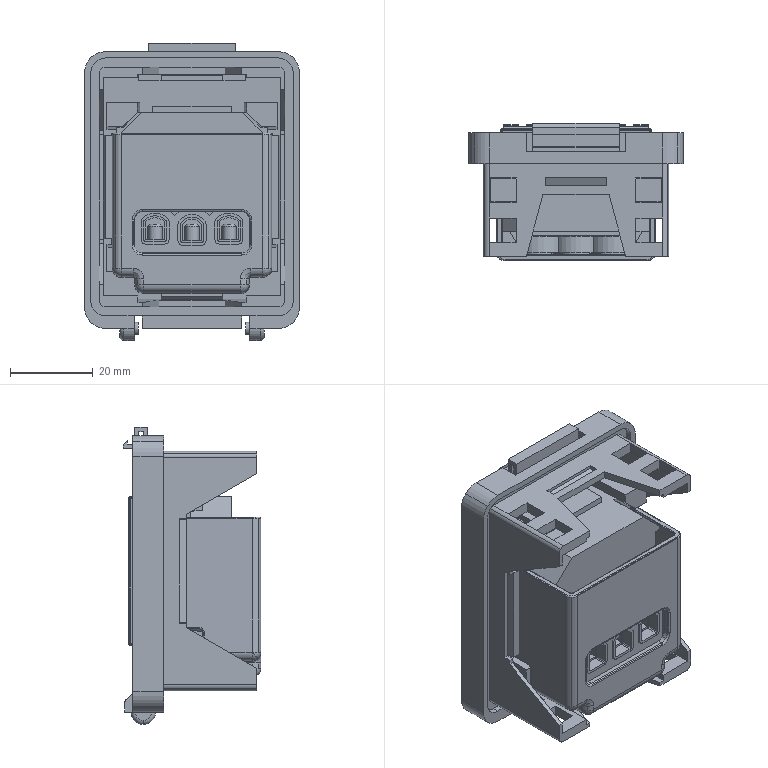Part | SolidWorks | features BaseBody 12 | 11 solids | 892 faces | box 52 x 33.3 x 71.95 mm | volume 53395 mm3 | plane 490 | cylinder 324 | spline 28 | sphere 18 | torus 16 | cone 16 | commonest cylinder face diameters 1 x114 0.6 x64 4.2 x26 4 x20 2.3 x12 3 x10